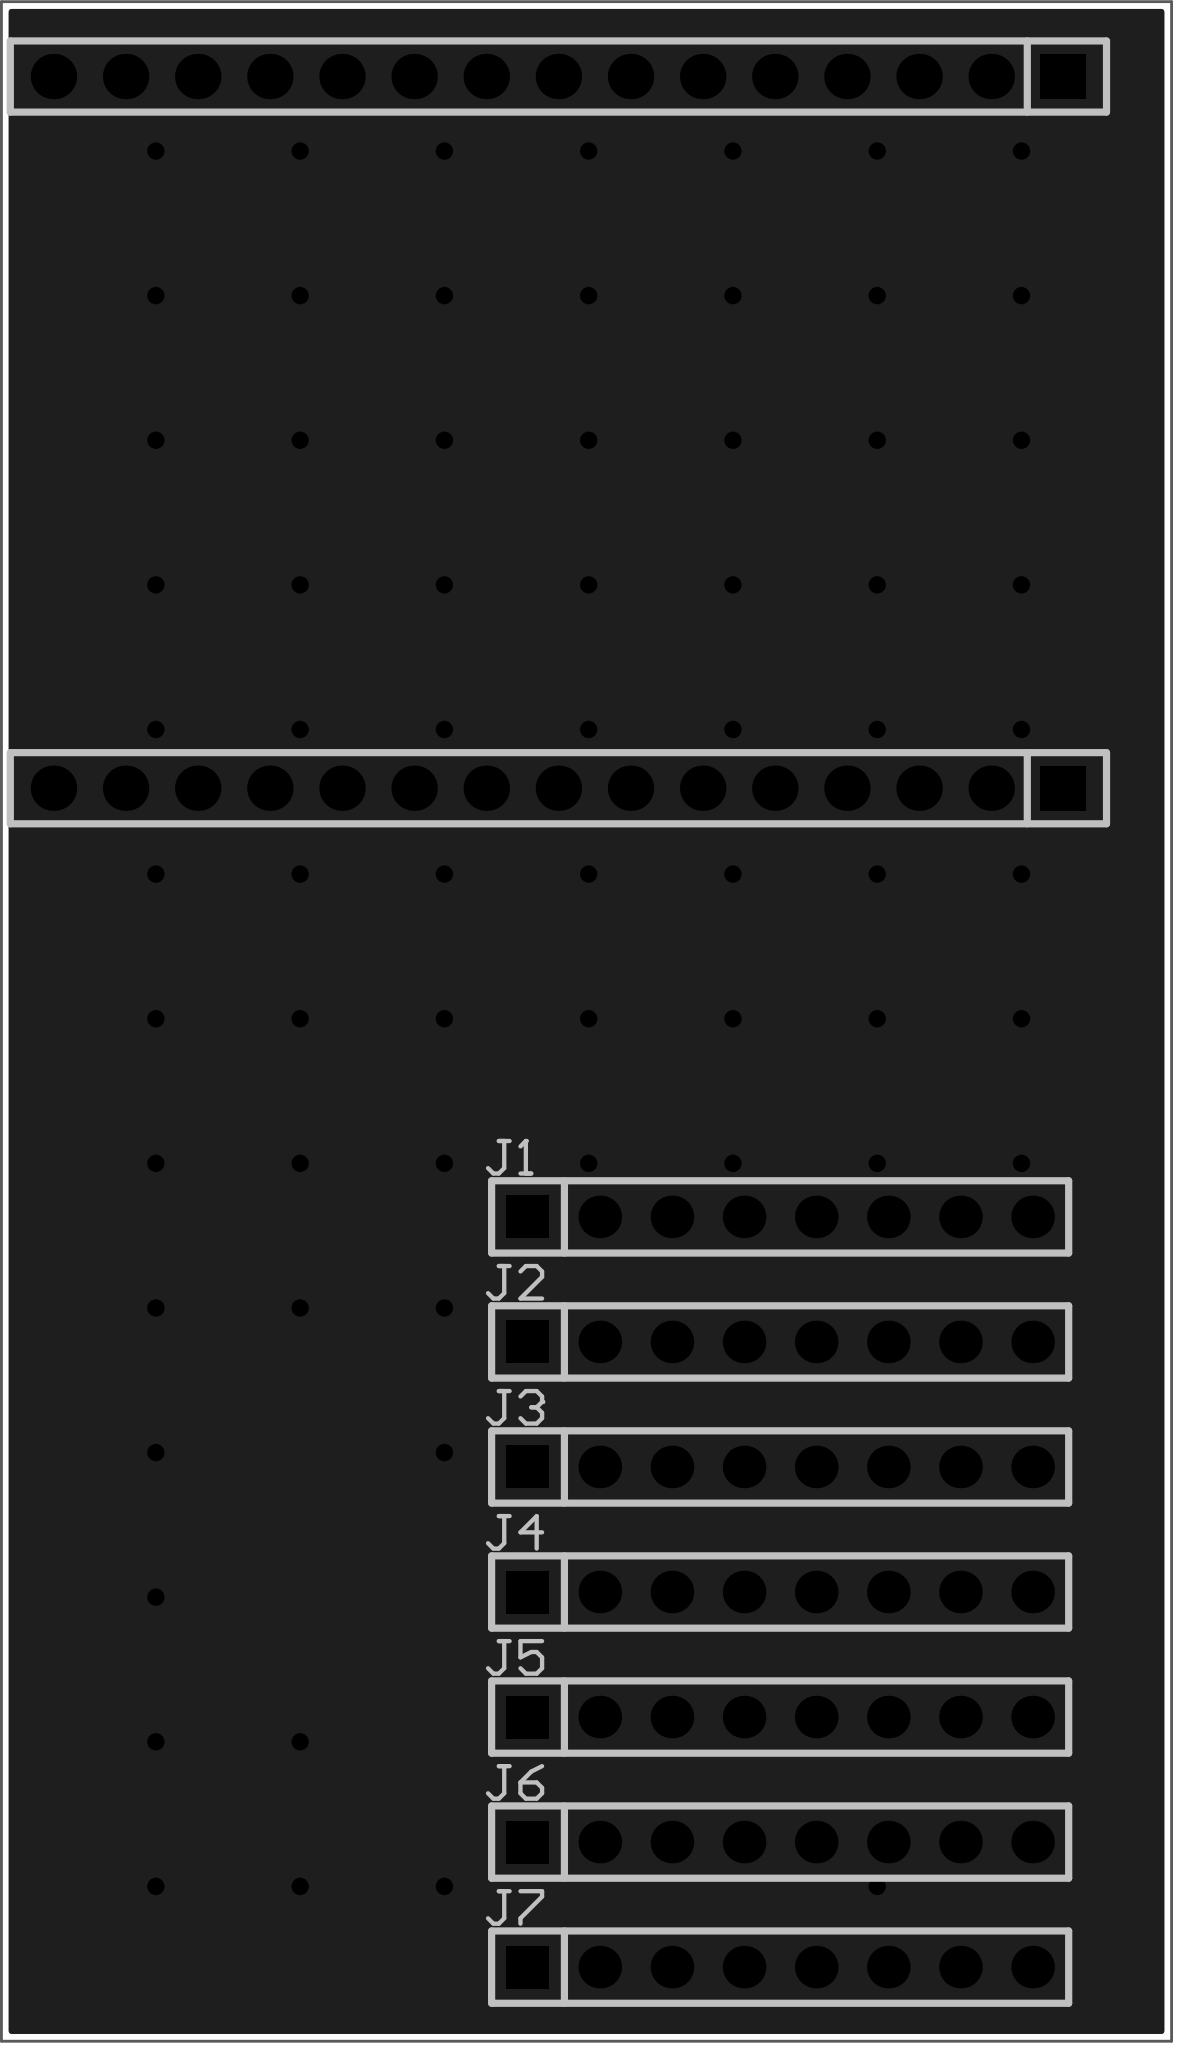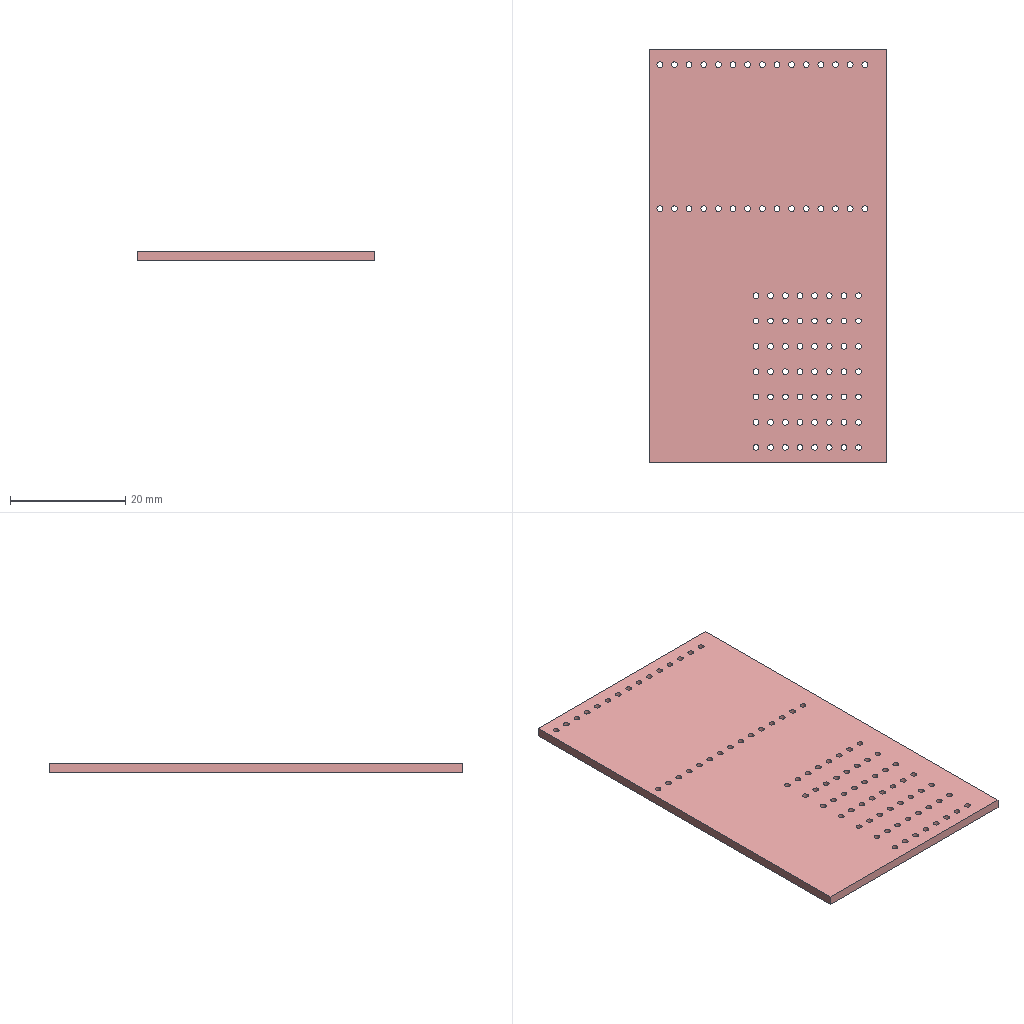Circuit board layout | Altium Designer | box 41.2 x 71.6 x 1.6 mm
Layer stack:
# Altium Designer layer stack of  (unit mm; dielectric type: 0 none, 1 core, 2 prepreg, 3 surface material)
index,name,kind,layer,copper_thickness_mm,dielectric_type,dielectric_thickness_mm,dielectric_material,dielectric_constant
0,Top Paste Mask Layer,other,,,,,,
1,Top Silkscreen Layer,other,,,,,,
2,Top Solder Mask Layer,dielectric,,,3,0.01,,3.3
3,Top Layer,copper,Top Layer,0.035,,,,
4,Dielectric1,dielectric,,,3,1.51,FR4,4.5
5,Bottom Layer,copper,Bottom Layer,0.035,,,,
6,Bottom Solder Mask Layer,dielectric,,,3,0.01,,3.3
7,Bottom Silkscreen Layer,other,,,,,,
8,Bottom Paste Mask Layer,other,,,,,,
# drill layer pairs: low layer,high layer
drill_pair,Top Layer,Bottom Layer
Part placement:
Designator,Comment,Layer,Footprint,Center-X(mm),Center-Y(mm),Rotation
J1,,TopLayer,HDR-TH_8P-P2.54-V-M,107.938,109.982,0
J2,,TopLayer,HDR-TH_8P-P2.54-V-M,107.938,105.59,0
J3,,TopLayer,HDR-TH_8P-P2.54-V-M,107.938,101.198,0
J4,,TopLayer,HDR-TH_8P-P2.54-V-M,107.938,96.806,0
J5,,TopLayer,HDR-TH_8P-P2.54-V-M,107.938,92.414,0
J6,,TopLayer,HDR-TH_8P-P2.54-V-M,107.938,88.022,0
J7,,TopLayer,HDR-TH_8P-P2.54-V-M,107.938,83.629,0
H1,,TopLayer,HDR-TH_15P-P2.54-V-F-1,100.13,150.041,180
H2,,TopLayer,HDR-TH_15P-P2.54-V-F-1,100.13,125.041,180
Pad and via stacks:
# Altium Designer via and pad stacks of  (unit mm). Each distinct definition once, with the count of objects using it.
# via: kind,start_layer,end_layer,hole_mm,diameter_mm,mode(0 simple;1 top-mid-bottom;2 full stack),diameter_per_layer,count,example_net
# pad: kind,layer,hole_mm,hole_type(0 round;1 square;2 slot),plating,top_size,top_shape(1 round;2 rect;3 octagon;9 rounded rect),mid_size,bottom_size,mode,footprint,size_per_layer,count,example
pad,Multi-Layer,1,0,plated,1.5x1.5,2,1.5x1.5,1.5x1.5,0,HDR-TH_8P-P2.54-V-M,,7,J1.1
pad,Multi-Layer,1,0,plated,1.5x1.5,1,1.5x1.5,1.5x1.5,0,HDR-TH_8P-P2.54-V-M,,49,J1.2
pad,Multi-Layer,1,0,plated,1.6x1.6,1,1.6x1.6,1.6x1.6,0,HDR-TH_15P-P2.54-V-F-1,,28,H1.15
pad,Multi-Layer,1,0,plated,1.6x1.575,2,1.6x1.575,1.6x1.575,0,HDR-TH_15P-P2.54-V-F-1,,2,H1.1
via,Top Layer,Bottom Layer,0.3048,0.61,0,,68,GND
Copper pours:
name,layer,net,type(0 solid;1 hatched;2 none)
Bottom Layer-GND,Bottom Layer,GND,0
Top Layer-GND,Top Layer,GND,0